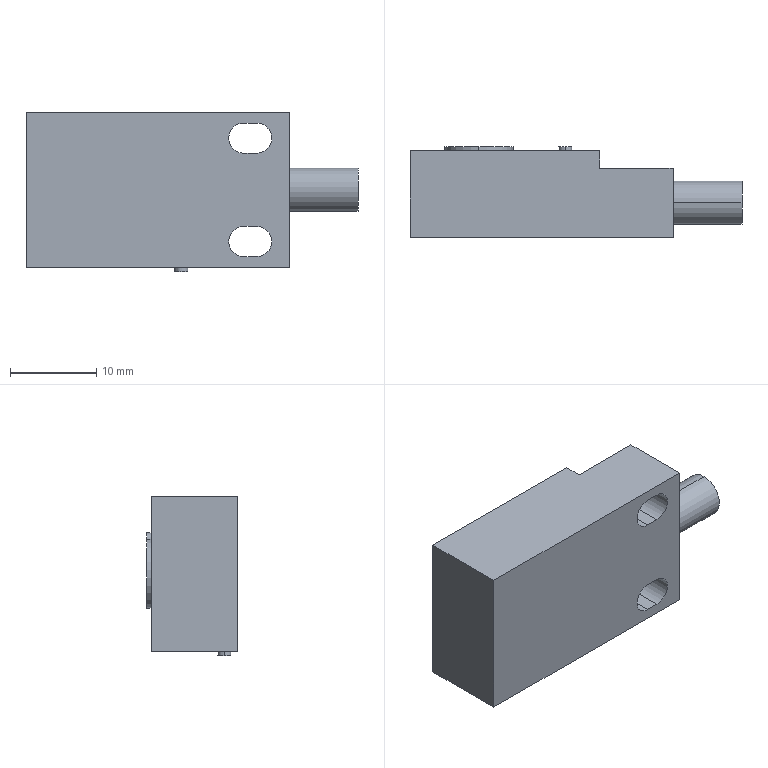Part | STEP file | Photoelectric proximity switch V1.201001 | 2 solids | 29 faces | box 38.5 x 10.5 x 18.5 mm | volume 5130 mm3 | plane 17 | cylinder 12 | commonest cylinder face diameters 1.5 x4 3.5 x4 5 x2 8 x2